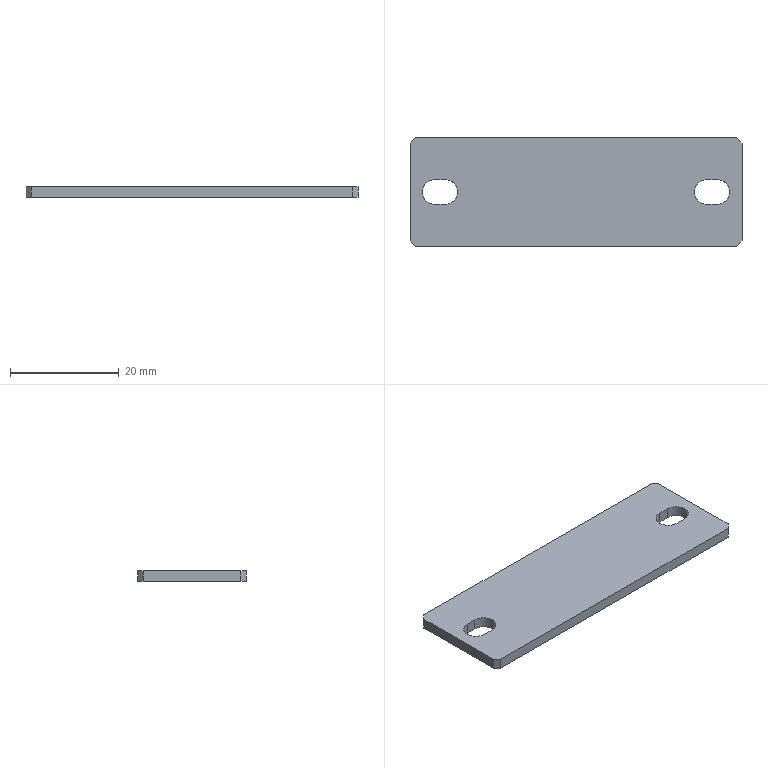Part | STEP file | 电源2 | 1 solid | 20 faces | box 61 x 20 x 2 mm | volume 2336 mm3 | plane 14 | cylinder 6 | commonest cylinder face diameters 4.5 x6